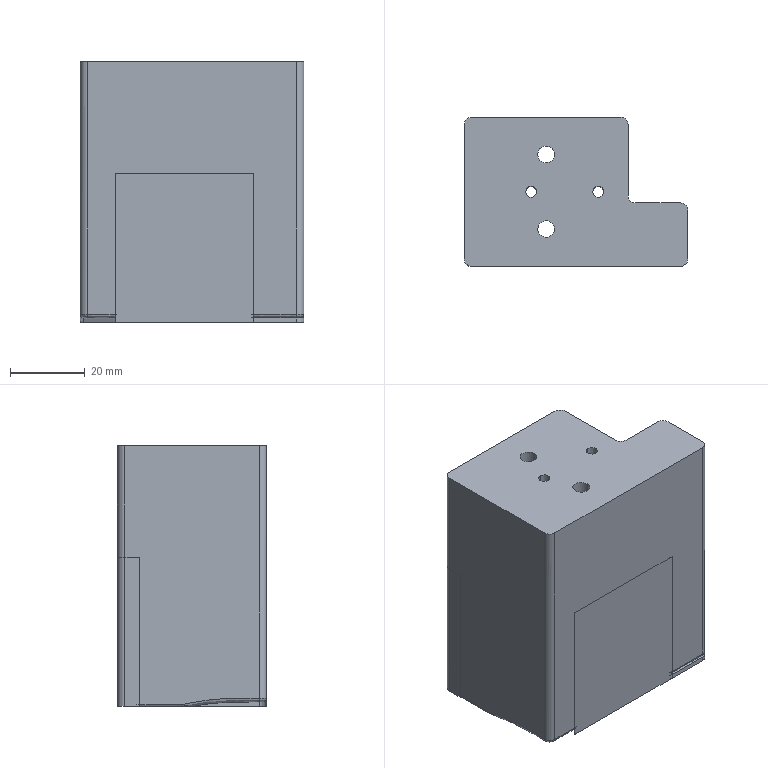NC program | NX | posted with a generic post | part box 60.004 x 40.015 x 70 mm
Lines 1 to 1043 of 35085:
N10 G17 G21 G94 G90
(FLOOR_WALL_2 , TOOL : D10)
N12 T09 M6
N14 G54
N16 G17 G0 G90 X3.828 Y-26.5 B0. C0. S9500 M3
N18 G43 Z30. H9
N20 Z0.503
N22 G94 G1 Z-0.998 F1000.
N24 X3.251 Y-25.5
N26 G3 X2.385 Y-25. R1.
N28 G1 X-28. F2500.
N30 G2 X-35. Y-18. R7.
N32 G1 Y-15.329
N34 X-34.97
N36 G3 X-29.689 Y-20.872 R7.1
N38 G1 X-28.989 Y-21.044
N40 X-28.097 Y-21.263
N42 G3 X-19.991 Y-19.799 R10.1
N44 G1 X-18.821 Y-18.938
N46 X-17.623 Y-17.875
N48 X-16.296 Y-16.425
N50 X-15.208 Y-14.922
N52 G3 X-13.539 Y-9.359 R10.1
N54 G1 X-13.563 Y18.5
N56 G3 X-19.19 Y24.97 R7.019
N58 G1 X15.05 Y25.
N60 Y24.97
N62 X14.897 Y24.953
N64 G3 X9.509 Y16.668 R7.077
N66 G1 X13.031 Y1.556
N68 X14.178 Y0.345
N70 X14.58 Y-0.08
N72 G3 X15.858 Y-1.059 R5.1
N74 G1 X16.454 Y-1.381
N76 G3 X18.053 Y-1.928 R5.1
N78 G1 X19. Y-2.083
N80 Y-18.
N82 G2 X12. Y-25. R7.
N84 G1 X2.385
N86 Y-20.
N88 X-12.789
N90 X-12.414 Y-19.59
N92 X-11.094 Y-17.766
N94 G3 X-8.539 Y-9.358 R15.1
N96 G1 Y18.251
N98 G3 X-8.563 Y18.741 R5.
N100 G1 X-8.687 Y20.
N102 X4.547
N104 X4.324 Y17.951
N106 X4.542 Y16.086
N108 G3 X4.639 Y15.533 R5.
N110 G1 X8.162 Y0.421
N112 G3 X9.401 Y-1.882 R5.
N114 G1 X10.95 Y-3.518
N116 G3 X13.48 Y-5.457 R10.1
N118 G1 X14. Y-5.739
N120 Y-18.
N122 G2 X12. Y-20. R2.
N124 G1 X2.385
N126 Y-15.
N128 X-4.346
N130 G3 X-3.539 Y-9.357 R20.1
N132 G1 Y15.
N134 X-0.351
N136 G3 X-0.23 Y14.397 R10.
N138 G1 X3.293 Y-0.714
N140 G3 X5.771 Y-5.32 R10.
N142 G1 X7.32 Y-6.956
N144 G3 X9. Y-8.482 R15.1
N146 G1 Y-15.
N148 X2.385
N150 Y-10.
N152 X1.453
N154 G3 X1.461 Y-9.357 R25.1
N156 G1 Y-7.99
N158 G3 X2.14 Y-8.758 R15.
N160 G1 X3.316 Y-10.
N162 X2.385
N164 G3 X1.519 Y-10.5 R1.
N166 G1 Z0.503
N168 G0 X3.814 Y-26.5 Z-0.495
N170 G1 Z-1.995 F1000.
N172 X3.237 Y-25.5
N174 G3 X2.371 Y-25. R1.
N176 G1 X-28. F2500.
N178 G2 X-35. Y-18. R7.
N180 G1 Y-15.329
N182 X-34.97
N184 G3 X-29.689 Y-20.872 R7.1
N186 G1 X-28.989 Y-21.044
N188 X-28.097 Y-21.263
N190 G3 X-19.991 Y-19.799 R10.1
N192 G1 X-18.821 Y-18.938
N194 X-17.623 Y-17.875
N196 X-16.296 Y-16.425
N198 X-15.208 Y-14.922
N200 G3 X-13.539 Y-9.359 R10.1
N202 G1 X-13.563 Y18.5
N204 G3 X-18.321 Y24.706 R6.939
N206 G1 X-18.562 Y24.82
N208 X-18.833 Y24.862
N210 X-19.19 Y24.97
N212 X15.05
N214 X14.485 Y24.808
N216 X13.386 Y24.423
N218 X13.086 Y24.233
N220 X12.904 Y24.158
N222 X12.641 Y23.953
N224 X12.032 Y23.569
N226 G3 X9.509 Y16.668 R7.053
N228 G1 X13.031 Y1.556
N230 X14. Y0.533
N232 G3 X16.281 Y-1.318 R7.1
N234 X19. Y-2.083 R7.102
N236 G1 Y-18.
N238 G2 X12. Y-25. R7.
N240 G1 X2.371
N242 Y-20.
N244 X-12.789
N246 X-12.414 Y-19.59
N248 X-11.094 Y-17.766
N250 G3 X-8.539 Y-9.358 R15.1
N252 G1 Y18.251
N254 G3 X-8.563 Y18.741 R5.
N256 G1 X-8.687 Y20.
N258 X4.547
N260 X4.324 Y17.951
N262 X4.542 Y16.086
N264 G3 X4.639 Y15.533 R5.
N266 G1 X8.162 Y0.421
N268 G3 X9.401 Y-1.882 R5.
N270 G1 X10.253 Y-2.782
N272 G3 X14. Y-5.768 R12.1
N274 G1 Y-18.
N276 G2 X12. Y-20. R2.
N278 G1 X2.371
N280 Y-15.
N282 X-4.346
N284 G3 X-3.539 Y-9.357 R20.1
N286 G1 Y15.
N288 X-0.351
N290 G3 X-0.23 Y14.397 R10.
N292 G1 X3.293 Y-0.714
N294 G3 X5.771 Y-5.32 R10.
N296 G1 X6.529 Y-6.121
N298 G3 X8.954 Y-8.446 R17.1
N300 G1 X9. Y-15.
N302 X2.371
N304 Y-10.
N306 X1.453
N308 G3 X1.461 Y-9.357 R25.1
N310 G1 Y-7.99
N312 G3 X2.14 Y-8.758 R15.
N314 G1 X2.818 Y-9.474
N316 G3 X3.289 Y-10. R22.1
N318 G1 X2.371
N320 G3 X1.505 Y-10.5 R1.
N322 G1 Z-0.495
N324 G0 X3.814 Y-26.5 Z-1.493
N326 G1 Z-2.993 F1000.
N328 X3.237 Y-25.5
N330 G3 X2.371 Y-25. R1.
N332 G1 X-28. F2500.
N334 G2 X-35. Y-18. R7.
N336 G1 Y-15.329
N338 X-34.97
N340 G3 X-29.689 Y-20.872 R7.1
N342 G1 X-28.989 Y-21.044
N344 X-28.097 Y-21.263
N346 G3 X-19.991 Y-19.799 R10.1
N348 G1 X-18.821 Y-18.938
N350 X-17.623 Y-17.875
N352 X-16.296 Y-16.425
N354 X-15.208 Y-14.922
N356 G3 X-13.539 Y-9.359 R10.1
N358 G1 X-13.551 Y18.411
N360 G3 X-13.619 Y19.063 R7.1
N362 G1 X-13.651 Y19.39
N364 X-13.746 Y19.704
N366 G3 X-13.961 Y20.412 R7.1
N368 G1 X-14.056 Y20.726
N370 X-14.211 Y21.016
N372 G3 X-14.56 Y21.668 R7.1
N374 G1 X-14.715 Y21.958
N376 X-14.923 Y22.212
N378 G3 X-15.392 Y22.784 R7.1
N380 G1 X-15.601 Y23.038
N382 X-15.855 Y23.246
N384 G3 X-16.426 Y23.715 R7.1
N386 G1 X-16.68 Y23.924
N388 X-16.97 Y24.079
N390 G3 X-17.622 Y24.427 R7.1
N392 G1 X-17.912 Y24.582
N394 X-18.227 Y24.678
N396 G3 X-18.934 Y24.892 R7.1
N398 G1 X-19.19 Y24.97
N400 X15.05 Y25.
N402 Y24.97
N404 X14.897 Y24.953
N406 X14.541 Y24.828
N408 G3 X13.742 Y24.547 R7.1
N410 G1 X13.386 Y24.423
N412 X13.067 Y24.221
N414 G3 X12.351 Y23.77 R7.1
N416 G1 X12.032 Y23.569
N418 X11.765 Y23.301
N420 G3 X11.168 Y22.701 R7.1
N422 G1 X10.902 Y22.434
N424 X10.702 Y22.114
N426 G3 X10.253 Y21.396 R7.1
N428 G1 X10.053 Y21.076
N430 X9.93 Y20.72
N432 G3 X9.653 Y19.919 R7.1
N434 G1 X9.529 Y19.563
N436 X9.518 Y19.459
N438 X9.488 Y19.188
N440 G3 X9.397 Y18.346 R7.1
N442 G1 X9.356 Y17.971
N444 X9.4 Y17.596
N446 G3 X9.498 Y16.755 R7.1
N448 G1 X13.031 Y1.556
N450 X14. Y0.533
N452 G3 X17.25 Y-1.728 R7.1
N454 X19. Y-2.083 R7.102
N456 G1 Y-18.
N458 G2 X12. Y-25. R7.
N460 G1 X2.371
N462 Y-20.
N464 X-12.789
N466 X-12.414 Y-19.59
N468 X-11.094 Y-17.766
N470 G3 X-8.539 Y-9.358 R15.1
N472 G1 Y18.251
N474 G3 X-8.559 Y18.701 R5.
N476 X-8.654 Y19.665 R12.1
N478 G1 X-8.687 Y20.
N480 X4.547
N482 X4.532 Y19.858
N484 G3 X4.412 Y18.758 R12.1
N486 G1 X4.324 Y17.951
N488 X4.419 Y17.144
N490 G3 X4.548 Y16.041 R12.1
N492 X4.639 Y15.533 R5.
N494 G1 X8.162 Y0.421
N496 G3 X9.401 Y-1.882 R5.
N498 G1 X10.253 Y-2.782
N500 G3 X14. Y-5.768 R12.1
N502 G1 Y-18.
N504 G2 X12. Y-20. R2.
N506 G1 X2.371
N508 Y-15.
N510 X-4.346
N512 G3 X-3.539 Y-9.357 R20.1
N514 G1 Y15.
N516 X-0.351
N518 G3 X-0.23 Y14.397 R10.
N520 G1 X3.293 Y-0.714
N522 G3 X5.771 Y-5.32 R10.
N524 G1 X6.529 Y-6.121
N526 G3 X9. Y-8.482 R17.1
N528 G1 Y-15.
N530 X2.371
N532 Y-10.
N534 X1.453
N536 G3 X1.461 Y-9.357 R25.1
N538 G1 Y-7.99
N540 G3 X2.14 Y-8.758 R15.
N542 G1 X2.818 Y-9.474
N544 G3 X3.289 Y-10. R22.1
N546 G1 X2.371
N548 G3 X1.505 Y-10.5 R1.
N550 G1 Z-1.493
N552 G0 X3.814 Y-26.5 Z-2.49
N554 G1 Z-3.99 F1000.
N556 X3.237 Y-25.5
N558 G3 X2.371 Y-25. R1.
N560 G1 X-28. F2500.
N562 G2 X-35. Y-18. R7.
N564 G1 Y-15.329
N566 X-34.97
N568 G3 X-29.689 Y-20.872 R7.1
N570 G1 X-28.989 Y-21.044
N572 X-28.097 Y-21.263
N574 G3 X-19.991 Y-19.799 R10.1
N576 G1 X-18.821 Y-18.938
N578 X-17.623 Y-17.875
N580 X-16.296 Y-16.425
N582 X-15.208 Y-14.922
N584 G3 X-13.539 Y-9.359 R10.1
N586 G1 X-13.551 Y18.411
N588 G3 X-13.619 Y19.063 R7.1
N590 G1 X-13.651 Y19.39
N592 X-13.746 Y19.704
N594 G3 X-13.961 Y20.412 R7.1
N596 G1 X-14.056 Y20.726
N598 X-14.211 Y21.016
N600 G3 X-14.56 Y21.668 R7.1
N602 G1 X-14.715 Y21.958
N604 X-14.923 Y22.212
N606 G3 X-15.392 Y22.784 R7.1
N608 G1 X-15.601 Y23.038
N610 X-15.855 Y23.246
N612 G3 X-16.426 Y23.715 R7.1
N614 G1 X-16.68 Y23.924
N616 X-16.97 Y24.079
N618 G3 X-17.622 Y24.427 R7.1
N620 G1 X-17.912 Y24.582
N622 X-18.227 Y24.678
N624 G3 X-18.934 Y24.892 R7.1
N626 G1 X-19.19 Y24.97
N628 X15.05 Y25.
N630 Y24.97
N632 X14.897 Y24.953
N634 X14.541 Y24.828
N636 G3 X13.742 Y24.547 R7.1
N638 G1 X13.386 Y24.423
N640 X13.067 Y24.221
N642 G3 X12.351 Y23.77 R7.1
N644 G1 X12.032 Y23.569
N646 X11.765 Y23.301
N648 G3 X11.168 Y22.701 R7.1
N650 G1 X10.902 Y22.434
N652 X10.702 Y22.114
N654 G3 X10.253 Y21.396 R7.1
N656 G1 X10.053 Y21.076
N658 X9.93 Y20.72
N660 G3 X9.653 Y19.919 R7.1
N662 G1 X9.529 Y19.563
N664 X9.518 Y19.459
N666 X9.488 Y19.188
N668 G3 X9.397 Y18.346 R7.1
N670 G1 X9.356 Y17.971
N672 X9.4 Y17.596
N674 G3 X9.498 Y16.755 R7.1
N676 G1 X13.031 Y1.556
N678 X14. Y0.533
N680 G3 X16.281 Y-1.318 R7.1
N682 X19. Y-2.083 R7.102
N684 G1 Y-18.
N686 G2 X12. Y-25. R7.
N688 G1 X2.371
N690 Y-20.
N692 X-12.789
N694 X-12.414 Y-19.59
N696 X-11.094 Y-17.766
N698 G3 X-8.539 Y-9.358 R15.1
N700 G1 Y18.251
N702 G3 X-8.559 Y18.701 R5.
N704 X-8.654 Y19.665 R12.1
N706 G1 X-8.687 Y20.
N708 X4.547
N710 X4.532 Y19.858
N712 G3 X4.412 Y18.758 R12.1
N714 G1 X4.324 Y17.951
N716 X4.419 Y17.144
N718 G3 X4.548 Y16.041 R12.1
N720 X4.639 Y15.533 R5.
N722 G1 X8.162 Y0.421
N724 G3 X9.401 Y-1.882 R5.
N726 G1 X10.253 Y-2.782
N728 G3 X14. Y-5.768 R12.1
N730 G1 Y-18.
N732 G2 X12. Y-20. R2.
N734 G1 X2.371
N736 Y-15.
N738 X-4.346
N740 G3 X-3.539 Y-9.357 R20.1
N742 G1 Y15.
N744 X-0.351
N746 G3 X-0.23 Y14.397 R10.
N748 G1 X3.293 Y-0.714
N750 G3 X5.771 Y-5.32 R10.
N752 G1 X6.529 Y-6.121
N754 G3 X9. Y-8.482 R17.1
N756 G1 Y-15.
N758 X2.371
N760 Y-10.
N762 X1.453
N764 G3 X1.461 Y-9.357 R25.1
N766 G1 Y-7.99
N768 G3 X2.14 Y-8.758 R15.
N770 G1 X2.818 Y-9.474
N772 G3 X3.289 Y-10. R22.1
N774 G1 X2.371
N776 G3 X1.505 Y-10.5 R1.
N778 G1 Z-2.49
N780 G0 X3.814 Y-26.5 Z-3.488
N782 G1 Z-4.988 F1000.
N784 X3.237 Y-25.5
N786 G3 X2.371 Y-25. R1.
N788 G1 X-28. F2500.
N790 G2 X-35. Y-18. R7.
N792 G1 Y-15.329
N794 X-34.97
N796 G3 X-29.689 Y-20.872 R7.1
N798 G1 X-28.989 Y-21.044
N800 X-28.097 Y-21.263
N802 G3 X-19.991 Y-19.799 R10.1
N804 G1 X-18.821 Y-18.938
N806 X-17.623 Y-17.875
N808 X-16.296 Y-16.425
N810 X-15.208 Y-14.922
N812 G3 X-13.539 Y-9.359 R10.1
N814 G1 X-13.551 Y18.411
N816 G3 X-13.619 Y19.063 R7.1
N818 G1 X-13.651 Y19.39
N820 X-13.746 Y19.704
N822 G3 X-13.961 Y20.412 R7.1
N824 G1 X-14.056 Y20.726
N826 X-14.211 Y21.016
N828 G3 X-14.56 Y21.668 R7.1
N830 G1 X-14.715 Y21.958
N832 X-14.923 Y22.212
N834 G3 X-15.392 Y22.784 R7.1
N836 G1 X-15.601 Y23.038
N838 X-15.855 Y23.246
N840 G3 X-16.426 Y23.715 R7.1
N842 G1 X-16.68 Y23.924
N844 X-16.97 Y24.079
N846 G3 X-17.622 Y24.427 R7.1
N848 G1 X-17.912 Y24.582
N850 X-18.227 Y24.678
N852 G3 X-18.934 Y24.892 R7.1
N854 G1 X-19.19 Y24.97
N856 X15.05 Y25.
N858 Y24.97
N860 X14.897 Y24.953
N862 X14.541 Y24.828
N864 G3 X13.742 Y24.547 R7.1
N866 G1 X13.386 Y24.423
N868 X13.067 Y24.221
N870 G3 X12.351 Y23.77 R7.1
N872 G1 X12.032 Y23.569
N874 X11.765 Y23.301
N876 G3 X11.168 Y22.701 R7.1
N878 G1 X10.902 Y22.434
N880 X10.702 Y22.114
N882 G3 X10.253 Y21.396 R7.1
N884 G1 X10.053 Y21.076
N886 X9.93 Y20.72
N888 G3 X9.653 Y19.919 R7.1
N890 G1 X9.529 Y19.563
N892 X9.518 Y19.459
N894 X9.488 Y19.188
N896 G3 X9.397 Y18.346 R7.1
N898 G1 X9.356 Y17.971
N900 X9.4 Y17.596
N902 G3 X9.498 Y16.755 R7.1
N904 G1 X13.031 Y1.556
N906 X14. Y0.533
N908 G3 X16.281 Y-1.318 R7.1
N910 X19. Y-2.083 R7.102
N912 G1 Y-18.
N914 G2 X12. Y-25. R7.
N916 G1 X2.371
N918 Y-20.
N920 X-12.789
N922 X-12.414 Y-19.59
N924 X-11.094 Y-17.766
N926 G3 X-8.539 Y-9.358 R15.1
N928 G1 Y18.251
N930 G3 X-8.559 Y18.701 R5.
N932 X-8.654 Y19.665 R12.1
N934 G1 X-8.687 Y20.
N936 X4.547
N938 X4.532 Y19.858
N940 G3 X4.412 Y18.758 R12.1
N942 G1 X4.324 Y17.951
N944 X4.419 Y17.144
N946 G3 X4.548 Y16.041 R12.1
N948 X4.639 Y15.533 R5.
N950 G1 X8.162 Y0.421
N952 G3 X9.401 Y-1.882 R5.
N954 G1 X10.253 Y-2.782
N956 G3 X14. Y-5.768 R12.1
N958 G1 Y-18.
N960 G2 X12. Y-20. R2.
N962 G1 X2.371
N964 Y-15.
N966 X-4.346
N968 G3 X-3.539 Y-9.357 R20.1
N970 G1 Y15.
N972 X-0.351
N974 G3 X-0.23 Y14.397 R10.
N976 G1 X3.293 Y-0.714
N978 G3 X5.771 Y-5.32 R10.
N980 G1 X6.529 Y-6.121
N982 G3 X9. Y-8.482 R17.1
N984 G1 Y-15.
N986 X2.371
N988 Y-10.
N990 X1.453
N992 G3 X1.461 Y-9.357 R25.1
N994 G1 Y-7.99
N996 G3 X2.14 Y-8.758 R15.
N998 G1 X2.818 Y-9.474
N1000 G3 X3.289 Y-10. R22.1
N1002 G1 X2.371
N1004 G3 X1.505 Y-10.5 R1.
N1006 G1 Z-3.488
N1008 G0 X3.814 Y-26.5 Z-4.485
N1010 G1 Z-5.985 F1000.
N1012 X3.237 Y-25.5
N1014 G3 X2.371 Y-25. R1.
N1016 G1 X-28. F2500.
N1018 G2 X-35. Y-18. R7.
N1020 G1 Y-15.329
N1022 X-34.97
N1024 G3 X-29.689 Y-20.872 R7.1
N1026 G1 X-28.989 Y-21.044
N1028 X-28.097 Y-21.263
N1030 G3 X-19.991 Y-19.799 R10.1
N1032 G1 X-18.821 Y-18.938
N1034 X-17.623 Y-17.875
N1036 X-16.296 Y-16.425
N1038 X-15.208 Y-14.922
N1040 G3 X-13.539 Y-9.359 R10.1
N1042 G1 X-13.551 Y18.411
N1044 G3 X-13.619 Y19.063 R7.1
N1046 G1 X-13.651 Y19.39
N1048 X-13.746 Y19.704
N1050 G3 X-13.961 Y20.412 R7.1
N1052 G1 X-14.056 Y20.726
N1054 X-14.211 Y21.016
N1056 G3 X-14.56 Y21.668 R7.1
N1058 G1 X-14.715 Y21.958
N1060 X-14.923 Y22.212
N1062 G3 X-15.392 Y22.784 R7.1
N1064 G1 X-15.601 Y23.038
N1066 X-15.855 Y23.246
N1068 G3 X-16.426 Y23.715 R7.1
N1070 G1 X-16.68 Y23.924
N1072 X-16.97 Y24.079
N1074 G3 X-17.622 Y24.427 R7.1
N1076 G1 X-17.912 Y24.582
N1078 X-18.227 Y24.678
N1080 G3 X-18.934 Y24.892 R7.1
N1082 G1 X-19.19 Y24.97
N1084 X15.05 Y25.
N1086 Y24.97
N1088 X14.897 Y24.953
N1090 X14.541 Y24.828
N1092 G3 X13.742 Y24.547 R7.1
N1094 G1 X13.386 Y24.423
N1096 X13.067 Y24.221
N1098 G3 X12.351 Y23.77 R7.1
N1100 G1 X12.032 Y23.569
N1102 X11.765 Y23.301
N1104 G3 X11.168 Y22.701 R7.1
N1106 G1 X10.902 Y22.434
N1108 X10.702 Y22.114
N1110 G3 X10.253 Y21.396 R7.1
N1112 G1 X10.053 Y21.076
N1114 X9.93 Y20.72
N1116 G3 X9.653 Y19.919 R7.1
N1118 G1 X9.529 Y19.563
N1120 X9.518 Y19.459
N1122 X9.488 Y19.188
N1124 G3 X9.397 Y18.346 R7.1
N1126 G1 X9.356 Y17.971
N1128 X9.4 Y17.596
N1130 G3 X9.498 Y16.755 R7.1
N1132 G1 X13.031 Y1.556
N1134 X14. Y0.533
N1136 G3 X17.25 Y-1.728 R7.1
N1138 X19. Y-2.083 R7.102
N1140 G1 Y-18.
N1142 G2 X12. Y-25. R7.
N1144 G1 X2.371
N1146 Y-20.
N1148 X-12.789
N1150 X-12.414 Y-19.59
N1152 X-11.094 Y-17.766
N1154 G3 X-8.539 Y-9.358 R15.1
N1156 G1 Y18.251
N1158 G3 X-8.559 Y18.701 R5.
N1160 X-8.654 Y19.665 R12.1
N1162 G1 X-8.687 Y20.
N1164 X4.547
N1166 X4.532 Y19.858
N1168 G3 X4.412 Y18.758 R12.1
N1170 G1 X4.324 Y17.951
N1172 X4.419 Y17.144
N1174 G3 X4.548 Y16.041 R12.1
N1176 X4.639 Y15.533 R5.
N1178 G1 X8.162 Y0.421
N1180 G3 X9.401 Y-1.882 R5.
N1182 G1 X10.253 Y-2.782
N1184 G3 X14. Y-5.768 R12.1
N1186 G1 Y-18.
N1188 G2 X12. Y-20. R2.
N1190 G1 X2.371
N1192 Y-15.
N1194 X-4.346
N1196 G3 X-3.539 Y-9.357 R20.1
N1198 G1 Y15.
N1200 X-0.351
N1202 G3 X-0.23 Y14.397 R10.
N1204 G1 X3.293 Y-0.714
N1206 G3 X5.771 Y-5.32 R10.
N1208 G1 X6.529 Y-6.121
N1210 G3 X9. Y-8.482 R17.1
N1212 G1 Y-15.
N1214 X2.371
N1216 Y-10.
N1218 X1.453
N1220 G3 X1.461 Y-9.357 R25.1
N1222 G1 Y-7.99
N1224 G3 X2.14 Y-8.758 R15.
N1226 G1 X2.818 Y-9.474
N1228 G3 X3.289 Y-10. R22.1
N1230 G1 X2.371
N1232 G3 X1.505 Y-10.5 R1.
N1234 G1 Z-4.485
N1236 G0 X3.814 Y-26.5 Z-5.483
N1238 G1 Z-6.983 F1000.
N1240 X3.237 Y-25.5
N1242 G3 X2.371 Y-25. R1.
N1244 G1 X-28. F2500.
N1246 G2 X-35. Y-18. R7.
N1248 G1 Y-15.329
N1250 X-34.97
N1252 G3 X-29.689 Y-20.872 R7.1
N1254 G1 X-28.989 Y-21.044
N1256 X-28.097 Y-21.263
N1258 G3 X-19.991 Y-19.799 R10.1
N1260 G1 X-18.821 Y-18.938
N1262 X-17.623 Y-17.875
N1264 X-16.296 Y-16.425
N1266 X-15.208 Y-14.922
N1268 G3 X-13.539 Y-9.359 R10.1
N1270 G1 X-13.551 Y18.411
N1272 G3 X-13.619 Y19.063 R7.1
N1274 G1 X-13.651 Y19.39
N1276 X-13.746 Y19.704
N1278 G3 X-13.961 Y20.412 R7.1
N1280 G1 X-14.056 Y20.726
N1282 X-14.211 Y21.016
N1284 G3 X-14.56 Y21.668 R7.1
N1286 G1 X-14.715 Y21.958
N1288 X-14.923 Y22.212
N1290 G3 X-15.392 Y22.784 R7.1
N1292 G1 X-15.601 Y23.038
N1294 X-15.855 Y23.246
N1296 G3 X-16.426 Y23.715 R7.1
N1298 G1 X-16.68 Y23.924
N1300 X-16.97 Y24.079
N1302 G3 X-17.622 Y24.427 R7.1
N1304 G1 X-17.912 Y24.582
N1306 X-18.227 Y24.678
N1308 G3 X-18.934 Y24.892 R7.1
N1310 G1 X-19.19 Y24.97
N1312 X15.05 Y25.
N1314 Y24.97
N1316 X14.897 Y24.953
N1318 X14.541 Y24.828
N1320 G3 X13.742 Y24.547 R7.1
N1322 G1 X13.386 Y24.423
N1324 X13.067 Y24.221
N1326 G3 X12.351 Y23.77 R7.1
N1328 G1 X12.032 Y23.569
N1330 X11.765 Y23.301
N1332 G3 X11.168 Y22.701 R7.1
N1334 G1 X10.902 Y22.434
N1336 X10.702 Y22.114
N1338 G3 X10.253 Y21.396 R7.1
N1340 G1 X10.053 Y21.076
N1342 X9.93 Y20.72
N1344 G3 X9.653 Y19.919 R7.1
N1346 G1 X9.529 Y19.563
N1348 X9.518 Y19.459
N1350 X9.488 Y19.188
N1352 G3 X9.397 Y18.346 R7.1
N1354 G1 X9.356 Y17.971
N1356 X9.4 Y17.596
N1358 G3 X9.498 Y16.755 R7.1
N1360 G1 X13.031 Y1.556
N1362 X14. Y0.533
N1364 G3 X17.25 Y-1.728 R7.1
N1366 X19. Y-2.083 R7.102
N1368 G1 Y-18.
N1370 G2 X12. Y-25. R7.
N1372 G1 X2.371
N1374 Y-20.
N1376 X-12.789
N1378 X-12.414 Y-19.59
N1380 X-11.094 Y-17.766
N1382 G3 X-8.539 Y-9.358 R15.1
N1384 G1 Y18.251
N1386 G3 X-8.559 Y18.701 R5.
N1388 X-8.654 Y19.665 R12.1
N1390 G1 X-8.687 Y20.
N1392 X4.547
N1394 X4.532 Y19.858
N1396 G3 X4.412 Y18.758 R12.1
N1398 G1 X4.324 Y17.951
N1400 X4.419 Y17.144
N1402 G3 X4.548 Y16.041 R12.1
N1404 X4.639 Y15.533 R5.
N1406 G1 X8.162 Y0.421
N1408 G3 X9.401 Y-1.882 R5.
N1410 G1 X10.253 Y-2.782
N1412 G3 X14. Y-5.768 R12.1
N1414 G1 Y-18.
N1416 G2 X12. Y-20. R2.
N1418 G1 X2.371
N1420 Y-15.
N1422 X-4.346
N1424 G3 X-3.539 Y-9.357 R20.1
N1426 G1 Y15.
N1428 X-0.351
N1430 G3 X-0.23 Y14.397 R10.
N1432 G1 X3.293 Y-0.714
N1434 G3 X5.771 Y-5.32 R10.
N1436 G1 X6.529 Y-6.121
N1438 G3 X9. Y-8.482 R17.1
N1440 G1 Y-15.
N1442 X2.371
N1444 Y-10.
N1446 X1.453
N1448 G3 X1.461 Y-9.357 R25.1
N1450 G1 Y-7.99
N1452 G3 X2.14 Y-8.758 R15.
N1454 G1 X2.818 Y-9.474
N1456 G3 X3.289 Y-10. R22.1
N1458 G1 X2.371
N1460 G3 X1.505 Y-10.5 R1.
N1462 G1 Z-5.483
N1464 G0 X3.814 Y-26.5 Z-6.48
N1466 G1 Z-7.98 F1000.
N1468 X3.237 Y-25.5
N1470 G3 X2.371 Y-25. R1.
N1472 G1 X-28. F2500.
N1474 G2 X-35. Y-18. R7.
N1476 G1 Y-15.329
N1478 X-34.97
N1480 G3 X-29.689 Y-20.872 R7.1
N1482 G1 X-28.989 Y-21.044
N1484 X-28.097 Y-21.263
N1486 G3 X-19.991 Y-19.799 R10.1
N1488 G1 X-18.821 Y-18.938
N1490 X-17.623 Y-17.875
N1492 X-16.296 Y-16.425
N1494 X-15.208 Y-14.922
N1496 G3 X-13.539 Y-9.359 R10.1
N1498 G1 X-13.551 Y18.411
N1500 G3 X-13.619 Y19.063 R7.1
N1502 G1 X-13.651 Y19.39
N1504 X-13.746 Y19.704
N1506 G3 X-13.961 Y20.412 R7.1
N1508 G1 X-14.056 Y20.726
N1510 X-14.211 Y21.016
N1512 G3 X-14.56 Y21.668 R7.1
N1514 G1 X-14.715 Y21.958
N1516 X-14.923 Y22.212
N1518 G3 X-15.392 Y22.784 R7.1
N1520 G1 X-15.601 Y23.038
N1522 X-15.855 Y23.246
N1524 G3 X-16.426 Y23.715 R7.1
N1526 G1 X-16.68 Y23.924
N1528 X-16.97 Y24.079
N1530 G3 X-17.622 Y24.427 R7.1
N1532 G1 X-17.912 Y24.582
N1534 X-18.227 Y24.678
N1536 G3 X-18.934 Y24.892 R7.1
N1538 G1 X-19.19 Y24.97
N1540 X15.05 Y25.
N1542 Y24.97
N1544 X14.897 Y24.953
N1546 X14.541 Y24.828
N1548 G3 X13.742 Y24.547 R7.1
N1550 G1 X13.386 Y24.423
N1552 X13.067 Y24.221
N1554 G3 X12.351 Y23.77 R7.1
N1556 G1 X12.032 Y23.569
N1558 X11.765 Y23.301
N1560 G3 X11.168 Y22.701 R7.1
N1562 G1 X10.902 Y22.434
N1564 X10.702 Y22.114
N1566 G3 X10.253 Y21.396 R7.1
N1568 G1 X10.053 Y21.076
N1570 X9.93 Y20.72
N1572 G3 X9.653 Y19.919 R7.1
N1574 G1 X9.529 Y19.563
N1576 X9.518 Y19.459
N1578 X9.488 Y19.188
N1580 G3 X9.397 Y18.346 R7.1
N1582 G1 X9.356 Y17.971
N1584 X9.4 Y17.596
N1586 G3 X9.498 Y16.755 R7.1
N1588 G1 X13.031 Y1.556
N1590 X14. Y0.533
N1592 G3 X16.281 Y-1.318 R7.1
N1594 X19. Y-2.083 R7.102
N1596 G1 Y-18.
N1598 G2 X12. Y-25. R7.
N1600 G1 X2.371
N1602 Y-20.
N1604 X-12.789
N1606 X-12.414 Y-19.59
N1608 X-11.094 Y-17.766
N1610 G3 X-8.539 Y-9.358 R15.1
N1612 G1 Y18.251
N1614 G3 X-8.559 Y18.701 R5.
N1616 X-8.654 Y19.665 R12.1
N1618 G1 X-8.687 Y20.
N1620 X4.547
N1622 X4.532 Y19.858
N1624 G3 X4.412 Y18.758 R12.1
N1626 G1 X4.324 Y17.951
N1628 X4.419 Y17.144
N1630 G3 X4.548 Y16.041 R12.1
N1632 X4.639 Y15.533 R5.
N1634 G1 X8.162 Y0.421
N1636 G3 X9.401 Y-1.882 R5.
N1638 G1 X10.253 Y-2.782
N1640 G3 X14. Y-5.768 R12.1
N1642 G1 Y-18.
N1644 G2 X12. Y-20. R2.
N1646 G1 X2.371
N1648 Y-15.
N1650 X-4.346
N1652 G3 X-3.539 Y-9.357 R20.1
N1654 G1 Y15.
N1656 X-0.351
N1658 G3 X-0.23 Y14.397 R10.
N1660 G1 X3.293 Y-0.714
N1662 G3 X5.771 Y-5.32 R10.
N1664 G1 X6.529 Y-6.121
N1666 G3 X9. Y-8.482 R17.1
N1668 G1 Y-15.
N1670 X2.371
N1672 Y-10.
N1674 X1.453
N1676 G3 X1.461 Y-9.357 R25.1
N1678 G1 Y-7.99
N1680 G3 X2.14 Y-8.758 R15.
N1682 G1 X2.818 Y-9.474
N1684 G3 X3.289 Y-10. R22.1
N1686 G1 X2.371
N1688 G3 X1.505 Y-10.5 R1.
N1690 G1 Z-6.48
N1692 G0 X3.814 Y-26.5 Z-7.478
N1694 G1 Z-8.978 F1000.
N1696 X3.237 Y-25.5
N1698 G3 X2.371 Y-25. R1.
N1700 G1 X-28. F2500.
N1702 G2 X-35. Y-18. R7.
N1704 G1 Y-15.329
N1706 X-34.97
N1708 G3 X-29.689 Y-20.872 R7.1
N1710 G1 X-28.989 Y-21.044
N1712 X-28.097 Y-21.263
N1714 G3 X-19.991 Y-19.799 R10.1
N1716 G1 X-18.821 Y-18.938
N1718 X-17.623 Y-17.875
N1720 X-16.296 Y-16.425
N1722 X-15.208 Y-14.922
N1724 G3 X-13.539 Y-9.359 R10.1
N1726 G1 X-13.551 Y18.411
N1728 G3 X-13.619 Y19.063 R7.1
N1730 G1 X-13.651 Y19.39
N1732 X-13.746 Y19.704
N1734 G3 X-13.961 Y20.412 R7.1
N1736 G1 X-14.056 Y20.726
N1738 X-14.211 Y21.016
N1740 G3 X-14.56 Y21.668 R7.1
N1742 G1 X-14.715 Y21.958
N1744 X-14.923 Y22.212
N1746 G3 X-15.392 Y22.784 R7.1
N1748 G1 X-15.601 Y23.038
N1750 X-15.855 Y23.246
N1752 G3 X-16.426 Y23.715 R7.1
N1754 G1 X-16.68 Y23.924
N1756 X-16.97 Y24.079
N1758 G3 X-17.622 Y24.427 R7.1
N1760 G1 X-17.912 Y24.582
N1762 X-18.227 Y24.678
N1764 G3 X-18.934 Y24.892 R7.1
N1766 G1 X-19.19 Y24.97
N1768 X15.05 Y25.
N1770 Y24.97
N1772 X14.897 Y24.953
N1774 X14.541 Y24.828
N1776 G3 X13.742 Y24.547 R7.1
N1778 G1 X13.386 Y24.423
N1780 X13.067 Y24.221
N1782 G3 X12.351 Y23.77 R7.1
N1784 G1 X12.032 Y23.569
N1786 X11.765 Y23.301
N1788 G3 X11.168 Y22.701 R7.1
N1790 G1 X10.902 Y22.434
N1792 X10.702 Y22.114
N1794 G3 X10.253 Y21.396 R7.1
N1796 G1 X10.053 Y21.076
N1798 X9.93 Y20.72
N1800 G3 X9.653 Y19.919 R7.1
N1802 G1 X9.529 Y19.563
N1804 X9.518 Y19.459
N1806 X9.488 Y19.188
N1808 G3 X9.397 Y18.346 R7.1
N1810 G1 X9.356 Y17.971
N1812 X9.4 Y17.596
N1814 G3 X9.498 Y16.755 R7.1
N1816 G1 X13.031 Y1.556
N1818 X14. Y0.533
N1820 G3 X16.281 Y-1.318 R7.1
N1822 X19. Y-2.083 R7.102
N1824 G1 Y-18.
N1826 G2 X12. Y-25. R7.
N1828 G1 X2.371
N1830 Y-20.
N1832 X-12.789
N1834 X-12.414 Y-19.59
N1836 X-11.094 Y-17.766
N1838 G3 X-8.539 Y-9.358 R15.1
N1840 G1 Y18.251
N1842 G3 X-8.559 Y18.701 R5.
N1844 X-8.654 Y19.665 R12.1
N1846 G1 X-8.687 Y20.
N1848 X4.547
N1850 X4.532 Y19.858
N1852 G3 X4.412 Y18.758 R12.1
N1854 G1 X4.324 Y17.951
N1856 X4.419 Y17.144
N1858 G3 X4.548 Y16.041 R12.1
N1860 X4.639 Y15.533 R5.
N1862 G1 X8.162 Y0.421
N1864 G3 X9.401 Y-1.882 R5.
N1866 G1 X10.253 Y-2.782
N1868 G3 X14. Y-5.768 R12.1
N1870 G1 Y-18.
N1872 G2 X12. Y-20. R2.
N1874 G1 X2.371
N1876 Y-15.
N1878 X-4.346
N1880 G3 X-3.539 Y-9.357 R20.1
N1882 G1 Y15.
N1884 X-0.351
N1886 G3 X-0.23 Y14.397 R10.
N1888 G1 X3.293 Y-0.714
N1890 G3 X5.771 Y-5.32 R10.
N1892 G1 X6.529 Y-6.121
N1894 G3 X9. Y-8.482 R17.1
N1896 G1 Y-15.
N1898 X2.371
N1900 Y-10.
N1902 X1.453
N1904 G3 X1.461 Y-9.357 R25.1
N1906 G1 Y-7.99
N1908 G3 X2.14 Y-8.758 R15.
N1910 G1 X2.818 Y-9.474
N1912 G3 X3.289 Y-10. R22.1
N1914 G1 X2.371
N1916 G3 X1.505 Y-10.5 R1.
N1918 G1 Z-7.478
N1920 G0 X3.814 Y-26.5 Z-8.475
N1922 G1 Z-9.975 F1000.
N1924 X3.237 Y-25.5
N1926 G3 X2.371 Y-25. R1.
N1928 G1 X-28. F2500.
N1930 G2 X-35. Y-18. R7.
N1932 G1 Y-15.329
N1934 X-34.97
N1936 G3 X-29.689 Y-20.872 R7.1
N1938 G1 X-28.989 Y-21.044
N1940 X-28.097 Y-21.263
N1942 G3 X-19.991 Y-19.799 R10.1
N1944 G1 X-18.821 Y-18.938
N1946 X-17.623 Y-17.875
N1948 X-16.296 Y-16.425
N1950 X-15.208 Y-14.922
N1952 G3 X-13.539 Y-9.359 R10.1
N1954 G1 X-13.551 Y18.411
N1956 G3 X-13.619 Y19.063 R7.1
N1958 G1 X-13.651 Y19.39
N1960 X-13.746 Y19.704
N1962 G3 X-13.961 Y20.412 R7.1
N1964 G1 X-14.056 Y20.726
N1966 X-14.211 Y21.016
N1968 G3 X-14.56 Y21.668 R7.1
N1970 G1 X-14.715 Y21.958
N1972 X-14.923 Y22.212
N1974 G3 X-15.392 Y22.784 R7.1
N1976 G1 X-15.601 Y23.038
N1978 X-15.855 Y23.246
N1980 G3 X-16.426 Y23.715 R7.1
N1982 G1 X-16.68 Y23.924
N1984 X-16.97 Y24.079
N1986 G3 X-17.622 Y24.427 R7.1
N1988 G1 X-17.912 Y24.582
N1990 X-18.227 Y24.678
N1992 G3 X-18.934 Y24.892 R7.1
N1994 G1 X-19.19 Y24.97
N1996 X15.05 Y25.
N1998 Y24.97
N2000 X14.897 Y24.953
N2002 X14.541 Y24.828
N2004 G3 X13.742 Y24.547 R7.1
N2006 G1 X13.386 Y24.423
N2008 X13.067 Y24.221
N2010 G3 X12.351 Y23.77 R7.1
N2012 G1 X12.032 Y23.569
N2014 X11.765 Y23.301
N2016 G3 X11.168 Y22.701 R7.1
N2018 G1 X10.902 Y22.434
N2020 X10.702 Y22.114
N2022 G3 X10.253 Y21.396 R7.1
N2024 G1 X10.053 Y21.076
N2026 X9.93 Y20.72
N2028 G3 X9.653 Y19.919 R7.1
N2030 G1 X9.529 Y19.563
N2032 X9.518 Y19.459
N2034 X9.488 Y19.188
N2036 G3 X9.397 Y18.346 R7.1
N2038 G1 X9.356 Y17.971
N2040 X9.4 Y17.596
N2042 G3 X9.498 Y16.755 R7.1
N2044 G1 X13.031 Y1.556
N2046 X14. Y0.533
N2048 G3 X16.281 Y-1.318 R7.1
N2050 X19. Y-2.083 R7.102
N2052 G1 Y-18.
N2054 G2 X12. Y-25. R7.
N2056 G1 X2.371
N2058 Y-20.
N2060 X-12.789
N2062 X-12.414 Y-19.59
N2064 X-11.094 Y-17.766
N2066 G3 X-8.539 Y-9.358 R15.1
N2068 G1 Y18.251
N2070 G3 X-8.559 Y18.701 R5.
N2072 X-8.654 Y19.665 R12.1
N2074 G1 X-8.687 Y20.
N2076 X4.547
N2078 X4.532 Y19.858
N2080 G3 X4.412 Y18.758 R12.1
N2082 G1 X4.324 Y17.951
N2084 X4.419 Y17.144